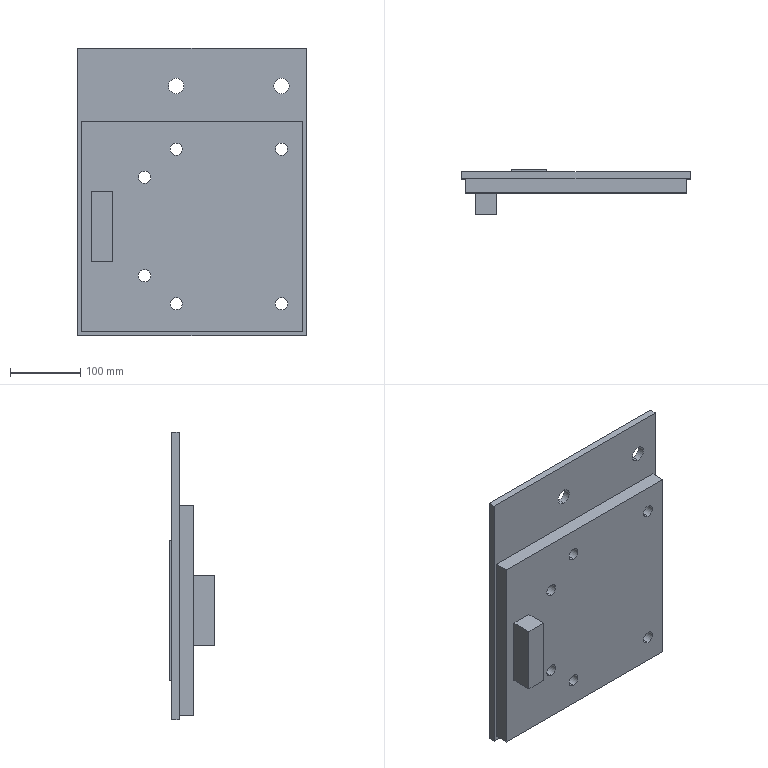Part | SolidWorks | features MirrorStock 1 | 4 solids | 56 faces | box 325 x 63 x 410 mm | volume 3290159 mm3 | cylinder 32 | plane 24 | commonest cylinder face diameters 17.5 x28 22 x4